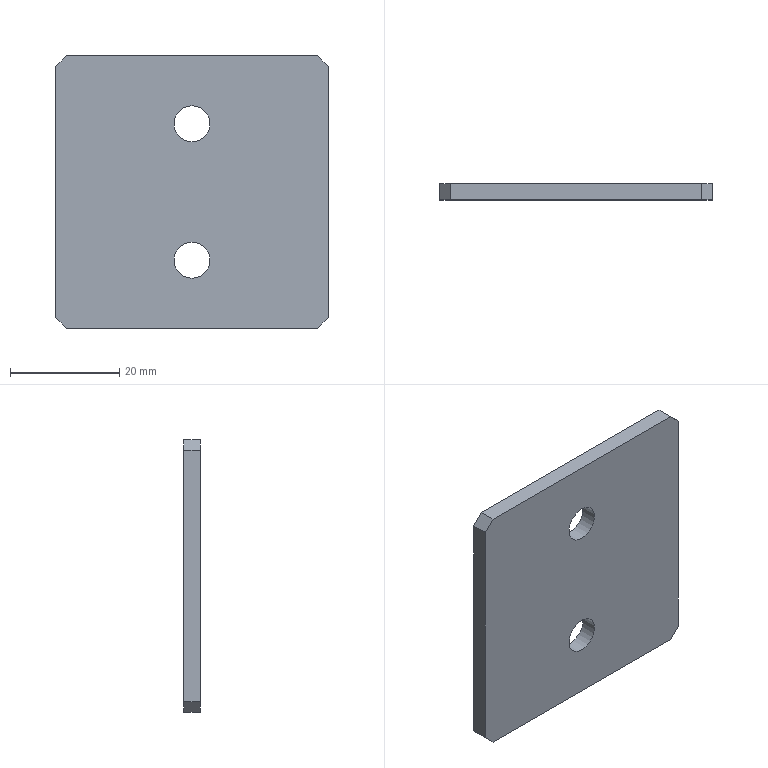Part | NX | 1 solid | 12 faces | box 50 x 3 x 50 mm | volume 7271 mm3 | plane 10 | cylinder 2 | commonest cylinder face diameters 6.6 x2
STEP:
#1=CARTESIAN_POINT('',(25.,0.,23.));
#2=VERTEX_POINT('',#1);
#3=CARTESIAN_POINT('',(25.,0.,-23.));
#4=VERTEX_POINT('',#3);
#5=CARTESIAN_POINT('',(25.,0.,25.));
#6=DIRECTION('',(0.,0.,-1.));
#7=VECTOR('',#6,1000.);
#8=LINE('',#5,#7);
#9=EDGE_CURVE('',#2,#4,#8,.T.);
#10=ORIENTED_EDGE('',*,*,#9,.T.);
#11=CARTESIAN_POINT('',(25.,3.,-23.));
#12=VERTEX_POINT('',#11);
#13=CARTESIAN_POINT('',(25.,3.,-23.));
#14=DIRECTION('',(0.,1.,0.));
#15=VECTOR('',#14,1000.);
#16=LINE('',#13,#15);
#17=EDGE_CURVE('',#4,#12,#16,.T.);
#18=ORIENTED_EDGE('',*,*,#17,.T.);
#19=CARTESIAN_POINT('',(25.,3.,23.));
#20=VERTEX_POINT('',#19);
#21=CARTESIAN_POINT('',(25.,3.,25.));
#22=DIRECTION('',(0.,0.,-1.));
#23=VECTOR('',#22,1000.);
#24=LINE('',#21,#23);
#25=EDGE_CURVE('',#20,#12,#24,.T.);
#26=ORIENTED_EDGE('',*,*,#25,.F.);
#27=CARTESIAN_POINT('',(25.,3.,23.));
#28=DIRECTION('',(0.,-1.,0.));
#29=VECTOR('',#28,1000.);
#30=LINE('',#27,#29);
#31=EDGE_CURVE('',#20,#2,#30,.T.);
#32=ORIENTED_EDGE('',*,*,#31,.T.);
#33=EDGE_LOOP('',(#10,#18,#26,#32));
#34=FACE_BOUND('',#33,.T.);
#35=CARTESIAN_POINT('',(25.,3.,25.));
#36=DIRECTION('',(-1.,0.,0.));
#37=DIRECTION('',(0.,0.,1.));
#38=AXIS2_PLACEMENT_3D('',#35,#36,#37);
#39=PLANE('',#38);
#40=ADVANCED_FACE('',(#34),#39,.F.);
#41=CARTESIAN_POINT('',(23.,0.,-25.));
#42=VERTEX_POINT('',#41);
#43=CARTESIAN_POINT('',(-23.,0.,-25.));
#44=VERTEX_POINT('',#43);
#45=CARTESIAN_POINT('',(-25.,0.,-25.));
#46=DIRECTION('',(-1.,0.,0.));
#47=VECTOR('',#46,1000.);
#48=LINE('',#45,#47);
#49=EDGE_CURVE('',#42,#44,#48,.T.);
#50=ORIENTED_EDGE('',*,*,#49,.T.);
#51=CARTESIAN_POINT('',(-23.,3.,-25.));
#52=VERTEX_POINT('',#51);
#53=CARTESIAN_POINT('',(-23.,3.,-25.));
#54=DIRECTION('',(0.,1.,0.));
#55=VECTOR('',#54,1000.);
#56=LINE('',#53,#55);
#57=EDGE_CURVE('',#44,#52,#56,.T.);
#58=ORIENTED_EDGE('',*,*,#57,.T.);
#59=CARTESIAN_POINT('',(23.,3.,-25.));
#60=VERTEX_POINT('',#59);
#61=CARTESIAN_POINT('',(-25.,3.,-25.));
#62=DIRECTION('',(-1.,0.,0.));
#63=VECTOR('',#62,1000.);
#64=LINE('',#61,#63);
#65=EDGE_CURVE('',#60,#52,#64,.T.);
#66=ORIENTED_EDGE('',*,*,#65,.F.);
#67=CARTESIAN_POINT('',(23.,3.,-25.));
#68=DIRECTION('',(0.,-1.,0.));
#69=VECTOR('',#68,1000.);
#70=LINE('',#67,#69);
#71=EDGE_CURVE('',#60,#42,#70,.T.);
#72=ORIENTED_EDGE('',*,*,#71,.T.);
#73=EDGE_LOOP('',(#50,#58,#66,#72));
#74=FACE_BOUND('',#73,.T.);
#75=CARTESIAN_POINT('',(-25.,3.,-25.));
#76=DIRECTION('',(0.,0.,1.));
#77=DIRECTION('',(1.,0.,0.));
#78=AXIS2_PLACEMENT_3D('',#75,#76,#77);
#79=PLANE('',#78);
#80=ADVANCED_FACE('',(#74),#79,.F.);
#81=CARTESIAN_POINT('',(-25.,0.,-23.));
#82=VERTEX_POINT('',#81);
#83=CARTESIAN_POINT('',(-25.,0.,23.));
#84=VERTEX_POINT('',#83);
#85=CARTESIAN_POINT('',(-25.,0.,25.));
#86=DIRECTION('',(0.,0.,1.));
#87=VECTOR('',#86,1000.);
#88=LINE('',#85,#87);
#89=EDGE_CURVE('',#82,#84,#88,.T.);
#90=ORIENTED_EDGE('',*,*,#89,.T.);
#91=CARTESIAN_POINT('',(-25.,3.,23.));
#92=VERTEX_POINT('',#91);
#93=CARTESIAN_POINT('',(-25.,3.,23.));
#94=DIRECTION('',(0.,1.,0.));
#95=VECTOR('',#94,1000.);
#96=LINE('',#93,#95);
#97=EDGE_CURVE('',#84,#92,#96,.T.);
#98=ORIENTED_EDGE('',*,*,#97,.T.);
#99=CARTESIAN_POINT('',(-25.,3.,-23.));
#100=VERTEX_POINT('',#99);
#101=CARTESIAN_POINT('',(-25.,3.,25.));
#102=DIRECTION('',(0.,0.,1.));
#103=VECTOR('',#102,1000.);
#104=LINE('',#101,#103);
#105=EDGE_CURVE('',#100,#92,#104,.T.);
#106=ORIENTED_EDGE('',*,*,#105,.F.);
#107=CARTESIAN_POINT('',(-25.,3.,-23.));
#108=DIRECTION('',(0.,-1.,0.));
#109=VECTOR('',#108,1000.);
#110=LINE('',#107,#109);
#111=EDGE_CURVE('',#100,#82,#110,.T.);
#112=ORIENTED_EDGE('',*,*,#111,.T.);
#113=EDGE_LOOP('',(#90,#98,#106,#112));
#114=FACE_BOUND('',#113,.T.);
#115=CARTESIAN_POINT('',(-25.,3.,25.));
#116=DIRECTION('',(1.,0.,0.));
#117=DIRECTION('',(0.,0.,-1.));
#118=AXIS2_PLACEMENT_3D('',#115,#116,#117);
#119=PLANE('',#118);
#120=ADVANCED_FACE('',(#114),#119,.F.);
#121=CARTESIAN_POINT('',(-23.,3.,25.));
#122=VERTEX_POINT('',#121);
#123=CARTESIAN_POINT('',(23.,3.,25.));
#124=VERTEX_POINT('',#123);
#125=CARTESIAN_POINT('',(-25.,3.,25.));
#126=DIRECTION('',(1.,0.,0.));
#127=VECTOR('',#126,1000.);
#128=LINE('',#125,#127);
#129=EDGE_CURVE('',#122,#124,#128,.T.);
#130=ORIENTED_EDGE('',*,*,#129,.F.);
#131=CARTESIAN_POINT('',(-23.,0.,25.));
#132=VERTEX_POINT('',#131);
#133=CARTESIAN_POINT('',(-23.,3.,25.));
#134=DIRECTION('',(0.,-1.,0.));
#135=VECTOR('',#134,1000.);
#136=LINE('',#133,#135);
#137=EDGE_CURVE('',#122,#132,#136,.T.);
#138=ORIENTED_EDGE('',*,*,#137,.T.);
#139=CARTESIAN_POINT('',(23.,0.,25.));
#140=VERTEX_POINT('',#139);
#141=CARTESIAN_POINT('',(-25.,0.,25.));
#142=DIRECTION('',(1.,0.,0.));
#143=VECTOR('',#142,1000.);
#144=LINE('',#141,#143);
#145=EDGE_CURVE('',#132,#140,#144,.T.);
#146=ORIENTED_EDGE('',*,*,#145,.T.);
#147=CARTESIAN_POINT('',(23.,3.,25.));
#148=DIRECTION('',(0.,1.,0.));
#149=VECTOR('',#148,1000.);
#150=LINE('',#147,#149);
#151=EDGE_CURVE('',#140,#124,#150,.T.);
#152=ORIENTED_EDGE('',*,*,#151,.T.);
#153=EDGE_LOOP('',(#130,#138,#146,#152));
#154=FACE_BOUND('',#153,.T.);
#155=CARTESIAN_POINT('',(-25.,3.,25.));
#156=DIRECTION('',(0.,0.,-1.));
#157=DIRECTION('',(-1.,0.,0.));
#158=AXIS2_PLACEMENT_3D('',#155,#156,#157);
#159=PLANE('',#158);
#160=ADVANCED_FACE('',(#154),#159,.F.);
#161=CARTESIAN_POINT('',(0.,3.,-9.2));
#162=VERTEX_POINT('',#161);
#163=CARTESIAN_POINT('',(0.,3.,-12.5));
#164=DIRECTION('',(0.,1.,0.));
#165=DIRECTION('',(0.,0.,1.));
#166=AXIS2_PLACEMENT_3D('',#163,#164,#165);
#167=CIRCLE('',#166,3.3);
#168=EDGE_CURVE('',#162,#162,#167,.T.);
#169=ORIENTED_EDGE('',*,*,#168,.F.);
#170=EDGE_LOOP('',(#169));
#171=FACE_BOUND('',#170,.T.);
#172=CARTESIAN_POINT('',(0.,3.,15.8));
#173=VERTEX_POINT('',#172);
#174=CARTESIAN_POINT('',(0.,3.,12.5));
#175=DIRECTION('',(0.,1.,0.));
#176=DIRECTION('',(0.,0.,1.));
#177=AXIS2_PLACEMENT_3D('',#174,#175,#176);
#178=CIRCLE('',#177,3.3);
#179=EDGE_CURVE('',#173,#173,#178,.T.);
#180=ORIENTED_EDGE('',*,*,#179,.F.);
#181=EDGE_LOOP('',(#180));
#182=FACE_BOUND('',#181,.T.);
#183=ORIENTED_EDGE('',*,*,#105,.T.);
#184=CARTESIAN_POINT('',(-23.,3.,25.));
#185=DIRECTION('',(-0.7071,0.,-0.7071));
#186=VECTOR('',#185,1000.);
#187=LINE('',#184,#186);
#188=EDGE_CURVE('',#92,#122,#187,.F.);
#189=ORIENTED_EDGE('',*,*,#188,.T.);
#190=ORIENTED_EDGE('',*,*,#129,.T.);
#191=CARTESIAN_POINT('',(25.,3.,23.));
#192=DIRECTION('',(-0.7071,0.,0.7071));
#193=VECTOR('',#192,1000.);
#194=LINE('',#191,#193);
#195=EDGE_CURVE('',#124,#20,#194,.F.);
#196=ORIENTED_EDGE('',*,*,#195,.T.);
#197=ORIENTED_EDGE('',*,*,#25,.T.);
#198=CARTESIAN_POINT('',(23.,3.,-25.));
#199=DIRECTION('',(0.7071,0.,0.7071));
#200=VECTOR('',#199,1000.);
#201=LINE('',#198,#200);
#202=EDGE_CURVE('',#12,#60,#201,.F.);
#203=ORIENTED_EDGE('',*,*,#202,.T.);
#204=ORIENTED_EDGE('',*,*,#65,.T.);
#205=CARTESIAN_POINT('',(-25.,3.,-23.));
#206=DIRECTION('',(0.7071,0.,-0.7071));
#207=VECTOR('',#206,1000.);
#208=LINE('',#205,#207);
#209=EDGE_CURVE('',#52,#100,#208,.F.);
#210=ORIENTED_EDGE('',*,*,#209,.T.);
#211=EDGE_LOOP('',(#183,#189,#190,#196,#197,#203,#204,#210));
#212=FACE_BOUND('',#211,.T.);
#213=CARTESIAN_POINT('',(0.,3.,0.));
#214=DIRECTION('',(0.,-1.,0.));
#215=DIRECTION('',(0.,0.,-1.));
#216=AXIS2_PLACEMENT_3D('',#213,#214,#215);
#217=PLANE('',#216);
#218=ADVANCED_FACE('',(#171,#182,#212),#217,.F.);
#219=CARTESIAN_POINT('',(0.,0.,-9.2));
#220=VERTEX_POINT('',#219);
#221=CARTESIAN_POINT('',(0.,0.,-12.5));
#222=DIRECTION('',(0.,1.,0.));
#223=DIRECTION('',(0.,0.,1.));
#224=AXIS2_PLACEMENT_3D('',#221,#222,#223);
#225=CIRCLE('',#224,3.3);
#226=EDGE_CURVE('',#220,#220,#225,.T.);
#227=ORIENTED_EDGE('',*,*,#226,.T.);
#228=EDGE_LOOP('',(#227));
#229=FACE_BOUND('',#228,.T.);
#230=CARTESIAN_POINT('',(0.,0.,15.8));
#231=VERTEX_POINT('',#230);
#232=CARTESIAN_POINT('',(0.,0.,12.5));
#233=DIRECTION('',(0.,1.,0.));
#234=DIRECTION('',(0.,0.,1.));
#235=AXIS2_PLACEMENT_3D('',#232,#233,#234);
#236=CIRCLE('',#235,3.3);
#237=EDGE_CURVE('',#231,#231,#236,.T.);
#238=ORIENTED_EDGE('',*,*,#237,.T.);
#239=EDGE_LOOP('',(#238));
#240=FACE_BOUND('',#239,.T.);
#241=ORIENTED_EDGE('',*,*,#145,.F.);
#242=CARTESIAN_POINT('',(-24.,0.,24.));
#243=DIRECTION('',(0.7071,0.,0.7071));
#244=VECTOR('',#243,1000.);
#245=LINE('',#242,#244);
#246=EDGE_CURVE('',#132,#84,#245,.F.);
#247=ORIENTED_EDGE('',*,*,#246,.T.);
#248=ORIENTED_EDGE('',*,*,#89,.F.);
#249=CARTESIAN_POINT('',(-24.,0.,-24.));
#250=DIRECTION('',(-0.7071,0.,0.7071));
#251=VECTOR('',#250,1000.);
#252=LINE('',#249,#251);
#253=EDGE_CURVE('',#82,#44,#252,.F.);
#254=ORIENTED_EDGE('',*,*,#253,.T.);
#255=ORIENTED_EDGE('',*,*,#49,.F.);
#256=CARTESIAN_POINT('',(24.,0.,-24.));
#257=DIRECTION('',(-0.7071,0.,-0.7071));
#258=VECTOR('',#257,1000.);
#259=LINE('',#256,#258);
#260=EDGE_CURVE('',#42,#4,#259,.F.);
#261=ORIENTED_EDGE('',*,*,#260,.T.);
#262=ORIENTED_EDGE('',*,*,#9,.F.);
#263=CARTESIAN_POINT('',(24.,0.,24.));
#264=DIRECTION('',(0.7071,0.,-0.7071));
#265=VECTOR('',#264,1000.);
#266=LINE('',#263,#265);
#267=EDGE_CURVE('',#2,#140,#266,.F.);
#268=ORIENTED_EDGE('',*,*,#267,.T.);
#269=EDGE_LOOP('',(#241,#247,#248,#254,#255,#261,#262,#268));
#270=FACE_BOUND('',#269,.T.);
#271=CARTESIAN_POINT('',(0.,0.,0.));
#272=DIRECTION('',(0.,-1.,0.));
#273=DIRECTION('',(0.,0.,-1.));
#274=AXIS2_PLACEMENT_3D('',#271,#272,#273);
#275=PLANE('',#274);
#276=ADVANCED_FACE('',(#229,#240,#270),#275,.T.);
#277=ORIENTED_EDGE('',*,*,#237,.F.);
#278=EDGE_LOOP('',(#277));
#279=FACE_BOUND('',#278,.T.);
#280=ORIENTED_EDGE('',*,*,#179,.T.);
#281=EDGE_LOOP('',(#280));
#282=FACE_BOUND('',#281,.T.);
#283=CARTESIAN_POINT('',(0.,3.,12.5));
#284=DIRECTION('',(0.,1.,0.));
#285=DIRECTION('',(0.,0.,1.));
#286=AXIS2_PLACEMENT_3D('',#283,#284,#285);
#287=CYLINDRICAL_SURFACE('',#286,3.3);
#288=ADVANCED_FACE('',(#279,#282),#287,.F.);
#289=ORIENTED_EDGE('',*,*,#226,.F.);
#290=EDGE_LOOP('',(#289));
#291=FACE_BOUND('',#290,.T.);
#292=ORIENTED_EDGE('',*,*,#168,.T.);
#293=EDGE_LOOP('',(#292));
#294=FACE_BOUND('',#293,.T.);
#295=CARTESIAN_POINT('',(0.,3.,-12.5));
#296=DIRECTION('',(0.,1.,0.));
#297=DIRECTION('',(0.,0.,1.));
#298=AXIS2_PLACEMENT_3D('',#295,#296,#297);
#299=CYLINDRICAL_SURFACE('',#298,3.3);
#300=ADVANCED_FACE('',(#291,#294),#299,.F.);
#301=ORIENTED_EDGE('',*,*,#188,.F.);
#302=ORIENTED_EDGE('',*,*,#97,.F.);
#303=ORIENTED_EDGE('',*,*,#246,.F.);
#304=ORIENTED_EDGE('',*,*,#137,.F.);
#305=EDGE_LOOP('',(#301,#302,#303,#304));
#306=FACE_BOUND('',#305,.T.);
#307=CARTESIAN_POINT('',(-23.,3.,25.));
#308=DIRECTION('',(0.7071,0.,-0.7071));
#309=DIRECTION('',(0.,-1.,0.));
#310=AXIS2_PLACEMENT_3D('',#307,#308,#309);
#311=PLANE('',#310);
#312=ADVANCED_FACE('',(#306),#311,.F.);
#313=ORIENTED_EDGE('',*,*,#209,.F.);
#314=ORIENTED_EDGE('',*,*,#57,.F.);
#315=ORIENTED_EDGE('',*,*,#253,.F.);
#316=ORIENTED_EDGE('',*,*,#111,.F.);
#317=EDGE_LOOP('',(#313,#314,#315,#316));
#318=FACE_BOUND('',#317,.T.);
#319=CARTESIAN_POINT('',(-25.,3.,-23.));
#320=DIRECTION('',(0.7071,0.,0.7071));
#321=DIRECTION('',(0.,-1.,0.));
#322=AXIS2_PLACEMENT_3D('',#319,#320,#321);
#323=PLANE('',#322);
#324=ADVANCED_FACE('',(#318),#323,.F.);
#325=ORIENTED_EDGE('',*,*,#202,.F.);
#326=ORIENTED_EDGE('',*,*,#17,.F.);
#327=ORIENTED_EDGE('',*,*,#260,.F.);
#328=ORIENTED_EDGE('',*,*,#71,.F.);
#329=EDGE_LOOP('',(#325,#326,#327,#328));
#330=FACE_BOUND('',#329,.T.);
#331=CARTESIAN_POINT('',(23.,3.,-25.));
#332=DIRECTION('',(-0.7071,0.,0.7071));
#333=DIRECTION('',(0.,-1.,0.));
#334=AXIS2_PLACEMENT_3D('',#331,#332,#333);
#335=PLANE('',#334);
#336=ADVANCED_FACE('',(#330),#335,.F.);
#337=ORIENTED_EDGE('',*,*,#195,.F.);
#338=ORIENTED_EDGE('',*,*,#151,.F.);
#339=ORIENTED_EDGE('',*,*,#267,.F.);
#340=ORIENTED_EDGE('',*,*,#31,.F.);
#341=EDGE_LOOP('',(#337,#338,#339,#340));
#342=FACE_BOUND('',#341,.T.);
#343=CARTESIAN_POINT('',(25.,3.,23.));
#344=DIRECTION('',(-0.7071,0.,-0.7071));
#345=DIRECTION('',(0.,-1.,0.));
#346=AXIS2_PLACEMENT_3D('',#343,#344,#345);
#347=PLANE('',#346);
#348=ADVANCED_FACE('',(#342),#347,.F.);
#349=CLOSED_SHELL('',(#40,#80,#120,#160,#218,#276,#288,#300,#312,#324,#336,#348));
#350=MANIFOLD_SOLID_BREP('',#349);
#351=(LENGTH_UNIT()NAMED_UNIT(*)SI_UNIT(.MILLI.,.METRE.));
#352=UNCERTAINTY_MEASURE_WITH_UNIT(LENGTH_MEASURE(0.00001),#351,'','');
#353=(NAMED_UNIT(*)PLANE_ANGLE_UNIT()SI_UNIT($,.RADIAN.));
#354=(NAMED_UNIT(*)SI_UNIT($,.STERADIAN.)SOLID_ANGLE_UNIT());
#355=(GEOMETRIC_REPRESENTATION_CONTEXT(3)GLOBAL_UNCERTAINTY_ASSIGNED_CONTEXT((#352))GLOBAL_UNIT_ASSIGNED_CONTEXT((#351,#353,#354))REPRESENTATION_CONTEXT('',''));
#356=ADVANCED_BREP_SHAPE_REPRESENTATION('',(#350),#355);